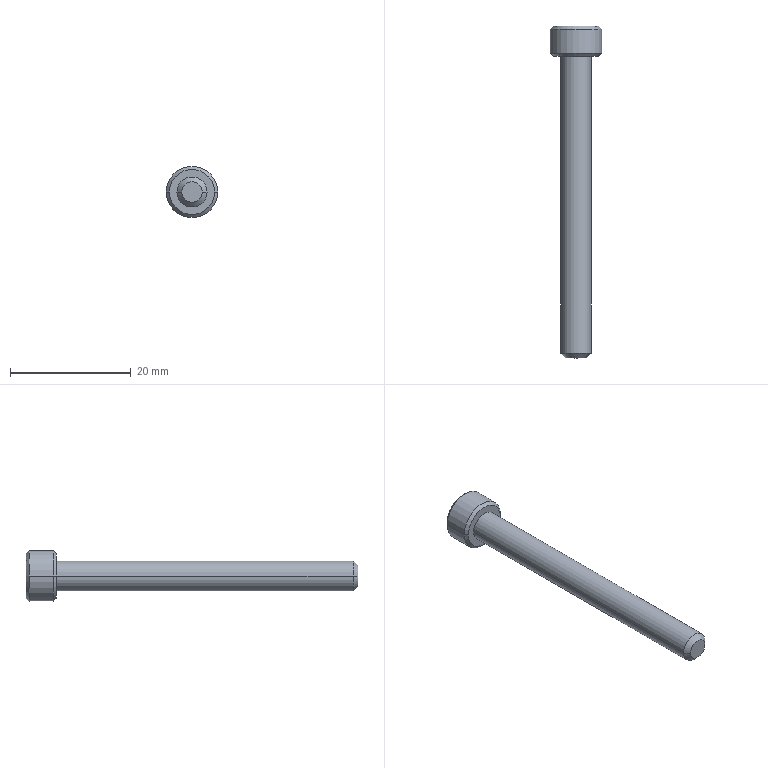Part | STEP file | BB62-M5-50L-14 | 1 solid | 27 faces | box 8.5 x 55 x 8.5 mm | volume 1213 mm3 | plane 15 | cone 8 | cylinder 4 | commonest cylinder face diameters 5 x2 8.5 x2
STEP:
#1=CARTESIAN_POINT('',(0.,1.178,0.));
#2=VERTEX_POINT('',#1);
#3=CARTESIAN_POINT('',(2.29,2.5,0.));
#4=VERTEX_POINT('',#3);
#5=CARTESIAN_POINT('',(0.,1.178,0.));
#6=DIRECTION('',(0.866,0.5,0.));
#7=VECTOR('',#6,1000.);
#8=LINE('',#5,#7);
#9=EDGE_CURVE('',#2,#4,#8,.T.);
#10=ORIENTED_EDGE('',*,*,#9,.F.);
#11=CARTESIAN_POINT('',(-2.29,2.5,0.));
#12=VERTEX_POINT('',#11);
#13=CARTESIAN_POINT('',(0.,1.178,0.));
#14=DIRECTION('',(-0.866,0.5,0.));
#15=VECTOR('',#14,1000.);
#16=LINE('',#13,#15);
#17=EDGE_CURVE('',#2,#12,#16,.T.);
#18=ORIENTED_EDGE('',*,*,#17,.T.);
#19=CARTESIAN_POINT('',(-1.983,2.5,1.145));
#20=VERTEX_POINT('',#19);
#21=CARTESIAN_POINT('',(0.,2.5,0.));
#22=DIRECTION('',(0.,-1.,0.));
#23=DIRECTION('',(-1.,0.,0.));
#24=AXIS2_PLACEMENT_3D('',#21,#22,#23);
#25=CIRCLE('',#24,2.29);
#26=EDGE_CURVE('',#20,#12,#25,.T.);
#27=ORIENTED_EDGE('',*,*,#26,.F.);
#28=CARTESIAN_POINT('',(0.,2.5,2.29));
#29=VERTEX_POINT('',#28);
#30=CARTESIAN_POINT('',(0.,2.5,0.));
#31=DIRECTION('',(0.,-1.,0.));
#32=DIRECTION('',(-1.,0.,0.));
#33=AXIS2_PLACEMENT_3D('',#30,#31,#32);
#34=CIRCLE('',#33,2.29);
#35=EDGE_CURVE('',#29,#20,#34,.T.);
#36=ORIENTED_EDGE('',*,*,#35,.F.);
#37=CARTESIAN_POINT('',(1.983,2.5,1.145));
#38=VERTEX_POINT('',#37);
#39=CARTESIAN_POINT('',(0.,2.5,0.));
#40=DIRECTION('',(0.,-1.,0.));
#41=DIRECTION('',(-1.,0.,0.));
#42=AXIS2_PLACEMENT_3D('',#39,#40,#41);
#43=CIRCLE('',#42,2.29);
#44=EDGE_CURVE('',#38,#29,#43,.T.);
#45=ORIENTED_EDGE('',*,*,#44,.F.);
#46=CARTESIAN_POINT('',(0.,2.5,0.));
#47=DIRECTION('',(0.,-1.,0.));
#48=DIRECTION('',(-1.,0.,0.));
#49=AXIS2_PLACEMENT_3D('',#46,#47,#48);
#50=CIRCLE('',#49,2.29);
#51=EDGE_CURVE('',#4,#38,#50,.T.);
#52=ORIENTED_EDGE('',*,*,#51,.F.);
#53=EDGE_LOOP('',(#10,#18,#27,#36,#45,#52));
#54=FACE_OUTER_BOUND('',#53,.T.);
#55=CARTESIAN_POINT('',(0.,1001.178,0.));
#56=DIRECTION('',(0.,1.,0.));
#57=DIRECTION('',(1.,0.,0.));
#58=AXIS2_PLACEMENT_3D('',#55,#56,#57);
#59=CONICAL_SURFACE('',#58,1732.051,1.047);
#60=ADVANCED_FACE('',(#54),#59,.F.);
#61=CARTESIAN_POINT('',(1.7,-50.,0.));
#62=VERTEX_POINT('',#61);
#63=CARTESIAN_POINT('',(-1.7,-50.,0.));
#64=VERTEX_POINT('',#63);
#65=CARTESIAN_POINT('',(0.,-50.,0.));
#66=DIRECTION('',(0.,1.,0.));
#67=DIRECTION('',(1.,0.,0.));
#68=AXIS2_PLACEMENT_3D('',#65,#66,#67);
#69=CIRCLE('',#68,1.7);
#70=EDGE_CURVE('',#62,#64,#69,.T.);
#71=ORIENTED_EDGE('',*,*,#70,.T.);
#72=CARTESIAN_POINT('',(-2.5,-49.2,0.));
#73=VERTEX_POINT('',#72);
#74=CARTESIAN_POINT('',(-1.7,-50.,0.));
#75=DIRECTION('',(-0.7071,0.7071,0.));
#76=VECTOR('',#75,1000.);
#77=LINE('',#74,#76);
#78=EDGE_CURVE('',#64,#73,#77,.T.);
#79=ORIENTED_EDGE('',*,*,#78,.T.);
#80=CARTESIAN_POINT('',(2.5,-49.2,0.));
#81=VERTEX_POINT('',#80);
#82=CARTESIAN_POINT('',(0.,-49.2,0.));
#83=DIRECTION('',(0.,-1.,0.));
#84=DIRECTION('',(-1.,0.,0.));
#85=AXIS2_PLACEMENT_3D('',#82,#83,#84);
#86=CIRCLE('',#85,2.5);
#87=EDGE_CURVE('',#73,#81,#86,.T.);
#88=ORIENTED_EDGE('',*,*,#87,.T.);
#89=CARTESIAN_POINT('',(1.7,-50.,0.));
#90=DIRECTION('',(0.7071,0.7071,0.));
#91=VECTOR('',#90,1000.);
#92=LINE('',#89,#91);
#93=EDGE_CURVE('',#62,#81,#92,.T.);
#94=ORIENTED_EDGE('',*,*,#93,.F.);
#95=EDGE_LOOP('',(#71,#79,#88,#94));
#96=FACE_OUTER_BOUND('',#95,.T.);
#97=CARTESIAN_POINT('',(0.,-50.,0.));
#98=DIRECTION('',(0.,1.,0.));
#99=DIRECTION('',(1.,0.,0.));
#100=AXIS2_PLACEMENT_3D('',#97,#98,#99);
#101=CONICAL_SURFACE('',#100,1.7,0.7854);
#102=ADVANCED_FACE('',(#96),#101,.T.);
#103=ORIENTED_EDGE('',*,*,#87,.F.);
#104=CARTESIAN_POINT('',(-2.5,0.,0.));
#105=VERTEX_POINT('',#104);
#106=CARTESIAN_POINT('',(-2.5,-49.2,0.));
#107=DIRECTION('',(0.,1.,0.));
#108=VECTOR('',#107,1000.);
#109=LINE('',#106,#108);
#110=EDGE_CURVE('',#73,#105,#109,.T.);
#111=ORIENTED_EDGE('',*,*,#110,.T.);
#112=CARTESIAN_POINT('',(2.5,0.,0.));
#113=VERTEX_POINT('',#112);
#114=CARTESIAN_POINT('',(0.,0.,0.));
#115=DIRECTION('',(0.,-1.,0.));
#116=DIRECTION('',(-1.,0.,0.));
#117=AXIS2_PLACEMENT_3D('',#114,#115,#116);
#118=CIRCLE('',#117,2.5);
#119=EDGE_CURVE('',#105,#113,#118,.T.);
#120=ORIENTED_EDGE('',*,*,#119,.T.);
#121=CARTESIAN_POINT('',(2.5,-49.2,0.));
#122=DIRECTION('',(0.,1.,0.));
#123=VECTOR('',#122,1000.);
#124=LINE('',#121,#123);
#125=EDGE_CURVE('',#81,#113,#124,.T.);
#126=ORIENTED_EDGE('',*,*,#125,.F.);
#127=EDGE_LOOP('',(#103,#111,#120,#126));
#128=FACE_OUTER_BOUND('',#127,.T.);
#129=CARTESIAN_POINT('',(0.,-49.2,0.));
#130=DIRECTION('',(0.,1.,0.));
#131=DIRECTION('',(1.,0.,0.));
#132=AXIS2_PLACEMENT_3D('',#129,#130,#131);
#133=CYLINDRICAL_SURFACE('',#132,2.5);
#134=ADVANCED_FACE('',(#128),#133,.T.);
#135=CARTESIAN_POINT('',(-3.75,5.,0.));
#136=VERTEX_POINT('',#135);
#137=CARTESIAN_POINT('',(3.75,5.,0.));
#138=VERTEX_POINT('',#137);
#139=CARTESIAN_POINT('',(0.,5.,0.));
#140=DIRECTION('',(0.,-1.,0.));
#141=DIRECTION('',(-1.,0.,0.));
#142=AXIS2_PLACEMENT_3D('',#139,#140,#141);
#143=CIRCLE('',#142,3.75);
#144=EDGE_CURVE('',#136,#138,#143,.T.);
#145=ORIENTED_EDGE('',*,*,#144,.T.);
#146=CARTESIAN_POINT('',(4.25,4.5,0.));
#147=VERTEX_POINT('',#146);
#148=CARTESIAN_POINT('',(4.25,4.5,0.));
#149=DIRECTION('',(0.7071,-0.7071,0.));
#150=VECTOR('',#149,1000.);
#151=LINE('',#148,#150);
#152=EDGE_CURVE('',#138,#147,#151,.T.);
#153=ORIENTED_EDGE('',*,*,#152,.T.);
#154=CARTESIAN_POINT('',(-4.25,4.5,0.));
#155=VERTEX_POINT('',#154);
#156=CARTESIAN_POINT('',(0.,4.5,0.));
#157=DIRECTION('',(0.,-1.,0.));
#158=DIRECTION('',(-1.,0.,0.));
#159=AXIS2_PLACEMENT_3D('',#156,#157,#158);
#160=CIRCLE('',#159,4.25);
#161=EDGE_CURVE('',#155,#147,#160,.T.);
#162=ORIENTED_EDGE('',*,*,#161,.F.);
#163=CARTESIAN_POINT('',(-4.25,4.5,0.));
#164=DIRECTION('',(-0.7071,-0.7071,0.));
#165=VECTOR('',#164,1000.);
#166=LINE('',#163,#165);
#167=EDGE_CURVE('',#136,#155,#166,.T.);
#168=ORIENTED_EDGE('',*,*,#167,.F.);
#169=EDGE_LOOP('',(#145,#153,#162,#168));
#170=FACE_OUTER_BOUND('',#169,.T.);
#171=CARTESIAN_POINT('',(0.,4.5,0.));
#172=DIRECTION('',(0.,-1.,0.));
#173=DIRECTION('',(-1.,0.,0.));
#174=AXIS2_PLACEMENT_3D('',#171,#172,#173);
#175=CONICAL_SURFACE('',#174,4.25,0.7854);
#176=ADVANCED_FACE('',(#170),#175,.T.);
#177=ORIENTED_EDGE('',*,*,#161,.T.);
#178=CARTESIAN_POINT('',(4.25,0.5,0.));
#179=VERTEX_POINT('',#178);
#180=CARTESIAN_POINT('',(4.25,1.62,0.));
#181=DIRECTION('',(0.,-1.,0.));
#182=VECTOR('',#181,1000.);
#183=LINE('',#180,#182);
#184=EDGE_CURVE('',#147,#179,#183,.T.);
#185=ORIENTED_EDGE('',*,*,#184,.T.);
#186=CARTESIAN_POINT('',(-4.25,0.5,0.));
#187=VERTEX_POINT('',#186);
#188=CARTESIAN_POINT('',(0.,0.5,0.));
#189=DIRECTION('',(0.,-1.,0.));
#190=DIRECTION('',(-1.,0.,0.));
#191=AXIS2_PLACEMENT_3D('',#188,#189,#190);
#192=CIRCLE('',#191,4.25);
#193=EDGE_CURVE('',#187,#179,#192,.T.);
#194=ORIENTED_EDGE('',*,*,#193,.F.);
#195=CARTESIAN_POINT('',(-4.25,1.62,0.));
#196=DIRECTION('',(0.,-1.,0.));
#197=VECTOR('',#196,1000.);
#198=LINE('',#195,#197);
#199=EDGE_CURVE('',#155,#187,#198,.T.);
#200=ORIENTED_EDGE('',*,*,#199,.F.);
#201=EDGE_LOOP('',(#177,#185,#194,#200));
#202=FACE_OUTER_BOUND('',#201,.T.);
#203=CARTESIAN_POINT('',(0.,1.62,0.));
#204=DIRECTION('',(0.,-1.,0.));
#205=DIRECTION('',(-1.,0.,0.));
#206=AXIS2_PLACEMENT_3D('',#203,#204,#205);
#207=CYLINDRICAL_SURFACE('',#206,4.25);
#208=ADVANCED_FACE('',(#202),#207,.T.);
#209=CARTESIAN_POINT('',(-3.75,0.,0.));
#210=VERTEX_POINT('',#209);
#211=CARTESIAN_POINT('',(3.75,0.,0.));
#212=VERTEX_POINT('',#211);
#213=CARTESIAN_POINT('',(0.,0.,0.));
#214=DIRECTION('',(0.,-1.,0.));
#215=DIRECTION('',(-1.,0.,0.));
#216=AXIS2_PLACEMENT_3D('',#213,#214,#215);
#217=CIRCLE('',#216,3.75);
#218=EDGE_CURVE('',#210,#212,#217,.T.);
#219=ORIENTED_EDGE('',*,*,#218,.F.);
#220=CARTESIAN_POINT('',(-3.75,0.,0.));
#221=DIRECTION('',(-0.7071,0.7071,0.));
#222=VECTOR('',#221,1000.);
#223=LINE('',#220,#222);
#224=EDGE_CURVE('',#210,#187,#223,.T.);
#225=ORIENTED_EDGE('',*,*,#224,.T.);
#226=ORIENTED_EDGE('',*,*,#193,.T.);
#227=CARTESIAN_POINT('',(3.75,0.,0.));
#228=DIRECTION('',(0.7071,0.7071,0.));
#229=VECTOR('',#228,1000.);
#230=LINE('',#227,#229);
#231=EDGE_CURVE('',#212,#179,#230,.T.);
#232=ORIENTED_EDGE('',*,*,#231,.F.);
#233=EDGE_LOOP('',(#219,#225,#226,#232));
#234=FACE_OUTER_BOUND('',#233,.T.);
#235=CARTESIAN_POINT('',(0.,0.,0.));
#236=DIRECTION('',(0.,1.,0.));
#237=DIRECTION('',(1.,0.,0.));
#238=AXIS2_PLACEMENT_3D('',#235,#236,#237);
#239=CONICAL_SURFACE('',#238,3.75,0.7854);
#240=ADVANCED_FACE('',(#234),#239,.T.);
#241=ORIENTED_EDGE('',*,*,#144,.F.);
#242=CARTESIAN_POINT('',(0.,5.,0.));
#243=DIRECTION('',(0.,-1.,0.));
#244=DIRECTION('',(-1.,0.,0.));
#245=AXIS2_PLACEMENT_3D('',#242,#243,#244);
#246=CIRCLE('',#245,3.75);
#247=EDGE_CURVE('',#138,#136,#246,.T.);
#248=ORIENTED_EDGE('',*,*,#247,.F.);
#249=EDGE_LOOP('',(#241,#248));
#250=FACE_OUTER_BOUND('',#249,.T.);
#251=CARTESIAN_POINT('',(0.,5.,-2.29));
#252=VERTEX_POINT('',#251);
#253=CARTESIAN_POINT('',(-1.983,5.,-1.145));
#254=VERTEX_POINT('',#253);
#255=CARTESIAN_POINT('',(0.,5.,-2.29));
#256=DIRECTION('',(-0.866,0.,0.5));
#257=VECTOR('',#256,1000.);
#258=LINE('',#255,#257);
#259=EDGE_CURVE('',#252,#254,#258,.T.);
#260=ORIENTED_EDGE('',*,*,#259,.F.);
#261=CARTESIAN_POINT('',(1.983,5.,-1.145));
#262=VERTEX_POINT('',#261);
#263=CARTESIAN_POINT('',(1.983,5.,-1.145));
#264=DIRECTION('',(-0.866,0.,-0.5));
#265=VECTOR('',#264,1000.);
#266=LINE('',#263,#265);
#267=EDGE_CURVE('',#262,#252,#266,.T.);
#268=ORIENTED_EDGE('',*,*,#267,.F.);
#269=CARTESIAN_POINT('',(1.983,5.,1.145));
#270=VERTEX_POINT('',#269);
#271=CARTESIAN_POINT('',(1.983,5.,1.145));
#272=DIRECTION('',(0.,0.,-1.));
#273=VECTOR('',#272,1000.);
#274=LINE('',#271,#273);
#275=EDGE_CURVE('',#270,#262,#274,.T.);
#276=ORIENTED_EDGE('',*,*,#275,.F.);
#277=CARTESIAN_POINT('',(0.,5.,2.29));
#278=VERTEX_POINT('',#277);
#279=CARTESIAN_POINT('',(0.,5.,2.29));
#280=DIRECTION('',(0.866,0.,-0.5));
#281=VECTOR('',#280,1000.);
#282=LINE('',#279,#281);
#283=EDGE_CURVE('',#278,#270,#282,.T.);
#284=ORIENTED_EDGE('',*,*,#283,.F.);
#285=CARTESIAN_POINT('',(-1.983,5.,1.145));
#286=VERTEX_POINT('',#285);
#287=CARTESIAN_POINT('',(-1.983,5.,1.145));
#288=DIRECTION('',(0.866,0.,0.5));
#289=VECTOR('',#288,1000.);
#290=LINE('',#287,#289);
#291=EDGE_CURVE('',#286,#278,#290,.T.);
#292=ORIENTED_EDGE('',*,*,#291,.F.);
#293=CARTESIAN_POINT('',(-1.983,5.,-1.145));
#294=DIRECTION('',(0.,0.,1.));
#295=VECTOR('',#294,1000.);
#296=LINE('',#293,#295);
#297=EDGE_CURVE('',#254,#286,#296,.T.);
#298=ORIENTED_EDGE('',*,*,#297,.F.);
#299=EDGE_LOOP('',(#260,#268,#276,#284,#292,#298));
#300=FACE_BOUND('',#299,.T.);
#301=CARTESIAN_POINT('',(3.75,5.,0.));
#302=DIRECTION('',(0.,1.,0.));
#303=DIRECTION('',(1.,0.,0.));
#304=AXIS2_PLACEMENT_3D('',#301,#302,#303);
#305=PLANE('',#304);
#306=ADVANCED_FACE('',(#250,#300),#305,.T.);
#307=CARTESIAN_POINT('',(0.,0.,0.));
#308=DIRECTION('',(0.,-1.,0.));
#309=DIRECTION('',(-1.,0.,0.));
#310=AXIS2_PLACEMENT_3D('',#307,#308,#309);
#311=CIRCLE('',#310,2.5);
#312=EDGE_CURVE('',#113,#105,#311,.T.);
#313=ORIENTED_EDGE('',*,*,#312,.F.);
#314=ORIENTED_EDGE('',*,*,#119,.F.);
#315=EDGE_LOOP('',(#313,#314));
#316=FACE_BOUND('',#315,.T.);
#317=CARTESIAN_POINT('',(0.,0.,0.));
#318=DIRECTION('',(0.,-1.,0.));
#319=DIRECTION('',(-1.,0.,0.));
#320=AXIS2_PLACEMENT_3D('',#317,#318,#319);
#321=CIRCLE('',#320,3.75);
#322=EDGE_CURVE('',#212,#210,#321,.T.);
#323=ORIENTED_EDGE('',*,*,#322,.T.);
#324=ORIENTED_EDGE('',*,*,#218,.T.);
#325=EDGE_LOOP('',(#323,#324));
#326=FACE_OUTER_BOUND('',#325,.T.);
#327=CARTESIAN_POINT('',(0.,0.,0.));
#328=DIRECTION('',(0.,-1.,0.));
#329=DIRECTION('',(-1.,0.,0.));
#330=AXIS2_PLACEMENT_3D('',#327,#328,#329);
#331=PLANE('',#330);
#332=ADVANCED_FACE('',(#316,#326),#331,.T.);
#333=ORIENTED_EDGE('',*,*,#224,.F.);
#334=ORIENTED_EDGE('',*,*,#322,.F.);
#335=ORIENTED_EDGE('',*,*,#231,.T.);
#336=CARTESIAN_POINT('',(0.,0.5,0.));
#337=DIRECTION('',(0.,-1.,0.));
#338=DIRECTION('',(-1.,0.,0.));
#339=AXIS2_PLACEMENT_3D('',#336,#337,#338);
#340=CIRCLE('',#339,4.25);
#341=EDGE_CURVE('',#179,#187,#340,.T.);
#342=ORIENTED_EDGE('',*,*,#341,.T.);
#343=EDGE_LOOP('',(#333,#334,#335,#342));
#344=FACE_OUTER_BOUND('',#343,.T.);
#345=CARTESIAN_POINT('',(0.,0.,0.));
#346=DIRECTION('',(0.,1.,0.));
#347=DIRECTION('',(1.,0.,0.));
#348=AXIS2_PLACEMENT_3D('',#345,#346,#347);
#349=CONICAL_SURFACE('',#348,3.75,0.7854);
#350=ADVANCED_FACE('',(#344),#349,.T.);
#351=ORIENTED_EDGE('',*,*,#184,.F.);
#352=CARTESIAN_POINT('',(0.,4.5,0.));
#353=DIRECTION('',(0.,-1.,0.));
#354=DIRECTION('',(-1.,0.,0.));
#355=AXIS2_PLACEMENT_3D('',#352,#353,#354);
#356=CIRCLE('',#355,4.25);
#357=EDGE_CURVE('',#147,#155,#356,.T.);
#358=ORIENTED_EDGE('',*,*,#357,.T.);
#359=ORIENTED_EDGE('',*,*,#199,.T.);
#360=ORIENTED_EDGE('',*,*,#341,.F.);
#361=EDGE_LOOP('',(#351,#358,#359,#360));
#362=FACE_OUTER_BOUND('',#361,.T.);
#363=CARTESIAN_POINT('',(0.,1.62,0.));
#364=DIRECTION('',(0.,-1.,0.));
#365=DIRECTION('',(-1.,0.,0.));
#366=AXIS2_PLACEMENT_3D('',#363,#364,#365);
#367=CYLINDRICAL_SURFACE('',#366,4.25);
#368=ADVANCED_FACE('',(#362),#367,.T.);
#369=ORIENTED_EDGE('',*,*,#152,.F.);
#370=ORIENTED_EDGE('',*,*,#247,.T.);
#371=ORIENTED_EDGE('',*,*,#167,.T.);
#372=ORIENTED_EDGE('',*,*,#357,.F.);
#373=EDGE_LOOP('',(#369,#370,#371,#372));
#374=FACE_OUTER_BOUND('',#373,.T.);
#375=CARTESIAN_POINT('',(0.,4.5,0.));
#376=DIRECTION('',(0.,-1.,0.));
#377=DIRECTION('',(-1.,0.,0.));
#378=AXIS2_PLACEMENT_3D('',#375,#376,#377);
#379=CONICAL_SURFACE('',#378,4.25,0.7854);
#380=ADVANCED_FACE('',(#374),#379,.T.);
#381=ORIENTED_EDGE('',*,*,#110,.F.);
#382=CARTESIAN_POINT('',(0.,-49.2,0.));
#383=DIRECTION('',(0.,-1.,0.));
#384=DIRECTION('',(-1.,0.,0.));
#385=AXIS2_PLACEMENT_3D('',#382,#383,#384);
#386=CIRCLE('',#385,2.5);
#387=EDGE_CURVE('',#81,#73,#386,.T.);
#388=ORIENTED_EDGE('',*,*,#387,.F.);
#389=ORIENTED_EDGE('',*,*,#125,.T.);
#390=ORIENTED_EDGE('',*,*,#312,.T.);
#391=EDGE_LOOP('',(#381,#388,#389,#390));
#392=FACE_OUTER_BOUND('',#391,.T.);
#393=CARTESIAN_POINT('',(0.,-49.2,0.));
#394=DIRECTION('',(0.,1.,0.));
#395=DIRECTION('',(1.,0.,0.));
#396=AXIS2_PLACEMENT_3D('',#393,#394,#395);
#397=CYLINDRICAL_SURFACE('',#396,2.5);
#398=ADVANCED_FACE('',(#392),#397,.T.);
#399=ORIENTED_EDGE('',*,*,#70,.F.);
#400=CARTESIAN_POINT('',(0.,-50.,0.));
#401=DIRECTION('',(0.,1.,0.));
#402=DIRECTION('',(1.,0.,0.));
#403=AXIS2_PLACEMENT_3D('',#400,#401,#402);
#404=CIRCLE('',#403,1.7);
#405=EDGE_CURVE('',#64,#62,#404,.T.);
#406=ORIENTED_EDGE('',*,*,#405,.F.);
#407=EDGE_LOOP('',(#399,#406));
#408=FACE_OUTER_BOUND('',#407,.T.);
#409=CARTESIAN_POINT('',(0.,-50.,0.));
#410=DIRECTION('',(0.,-1.,0.));
#411=DIRECTION('',(-1.,0.,0.));
#412=AXIS2_PLACEMENT_3D('',#409,#410,#411);
#413=PLANE('',#412);
#414=ADVANCED_FACE('',(#408),#413,.T.);
#415=ORIENTED_EDGE('',*,*,#78,.F.);
#416=ORIENTED_EDGE('',*,*,#405,.T.);
#417=ORIENTED_EDGE('',*,*,#93,.T.);
#418=ORIENTED_EDGE('',*,*,#387,.T.);
#419=EDGE_LOOP('',(#415,#416,#417,#418));
#420=FACE_OUTER_BOUND('',#419,.T.);
#421=CARTESIAN_POINT('',(0.,-50.,0.));
#422=DIRECTION('',(0.,1.,0.));
#423=DIRECTION('',(1.,0.,0.));
#424=AXIS2_PLACEMENT_3D('',#421,#422,#423);
#425=CONICAL_SURFACE('',#424,1.7,0.7854);
#426=ADVANCED_FACE('',(#420),#425,.T.);
#427=CARTESIAN_POINT('',(1.983,2.5,-1.145));
#428=VERTEX_POINT('',#427);
#429=CARTESIAN_POINT('',(0.,2.5,-2.29));
#430=VERTEX_POINT('',#429);
#431=CARTESIAN_POINT('',(1.983,2.5,-1.145));
#432=DIRECTION('',(-0.866,0.,-0.5));
#433=VECTOR('',#432,1000.);
#434=LINE('',#431,#433);
#435=EDGE_CURVE('',#428,#430,#434,.T.);
#436=ORIENTED_EDGE('',*,*,#435,.F.);
#437=CARTESIAN_POINT('',(1.983,5.,-1.145));
#438=DIRECTION('',(0.,-1.,0.));
#439=VECTOR('',#438,1000.);
#440=LINE('',#437,#439);
#441=EDGE_CURVE('',#262,#428,#440,.T.);
#442=ORIENTED_EDGE('',*,*,#441,.F.);
#443=ORIENTED_EDGE('',*,*,#267,.T.);
#444=CARTESIAN_POINT('',(0.,5.,-2.29));
#445=DIRECTION('',(0.,-1.,0.));
#446=VECTOR('',#445,1000.);
#447=LINE('',#444,#446);
#448=EDGE_CURVE('',#252,#430,#447,.T.);
#449=ORIENTED_EDGE('',*,*,#448,.T.);
#450=EDGE_LOOP('',(#436,#442,#443,#449));
#451=FACE_OUTER_BOUND('',#450,.T.);
#452=CARTESIAN_POINT('',(1.983,5.,-1.145));
#453=DIRECTION('',(-0.5,0.,0.866));
#454=DIRECTION('',(0.866,0.,0.5));
#455=AXIS2_PLACEMENT_3D('',#452,#453,#454);
#456=PLANE('',#455);
#457=ADVANCED_FACE('',(#451),#456,.T.);
#458=CARTESIAN_POINT('',(-1.983,2.5,-1.145));
#459=VERTEX_POINT('',#458);
#460=CARTESIAN_POINT('',(0.,2.5,-2.29));
#461=DIRECTION('',(-0.866,0.,0.5));
#462=VECTOR('',#461,1000.);
#463=LINE('',#460,#462);
#464=EDGE_CURVE('',#430,#459,#463,.T.);
#465=ORIENTED_EDGE('',*,*,#464,.F.);
#466=ORIENTED_EDGE('',*,*,#448,.F.);
#467=ORIENTED_EDGE('',*,*,#259,.T.);
#468=CARTESIAN_POINT('',(-1.983,5.,-1.145));
#469=DIRECTION('',(0.,-1.,0.));
#470=VECTOR('',#469,1000.);
#471=LINE('',#468,#470);
#472=EDGE_CURVE('',#254,#459,#471,.T.);
#473=ORIENTED_EDGE('',*,*,#472,.T.);
#474=EDGE_LOOP('',(#465,#466,#467,#473));
#475=FACE_OUTER_BOUND('',#474,.T.);
#476=CARTESIAN_POINT('',(0.,5.,-2.29));
#477=DIRECTION('',(0.5,0.,0.866));
#478=DIRECTION('',(0.866,0.,-0.5));
#479=AXIS2_PLACEMENT_3D('',#476,#477,#478);
#480=PLANE('',#479);
#481=ADVANCED_FACE('',(#475),#480,.T.);
#482=CARTESIAN_POINT('',(-1.983,2.5,-1.145));
#483=DIRECTION('',(0.,0.,1.));
#484=VECTOR('',#483,1000.);
#485=LINE('',#482,#484);
#486=EDGE_CURVE('',#459,#20,#485,.T.);
#487=ORIENTED_EDGE('',*,*,#486,.F.);
#488=ORIENTED_EDGE('',*,*,#472,.F.);
#489=ORIENTED_EDGE('',*,*,#297,.T.);
#490=CARTESIAN_POINT('',(-1.983,5.,1.145));
#491=DIRECTION('',(0.,-1.,0.));
#492=VECTOR('',#491,1000.);
#493=LINE('',#490,#492);
#494=EDGE_CURVE('',#286,#20,#493,.T.);
#495=ORIENTED_EDGE('',*,*,#494,.T.);
#496=EDGE_LOOP('',(#487,#488,#489,#495));
#497=FACE_OUTER_BOUND('',#496,.T.);
#498=CARTESIAN_POINT('',(-1.983,5.,-1.145));
#499=DIRECTION('',(1.,0.,0.));
#500=DIRECTION('',(0.,0.,-1.));
#501=AXIS2_PLACEMENT_3D('',#498,#499,#500);
#502=PLANE('',#501);
#503=ADVANCED_FACE('',(#497),#502,.T.);
#504=CARTESIAN_POINT('',(-1.983,2.5,1.145));
#505=DIRECTION('',(0.866,0.,0.5));
#506=VECTOR('',#505,1000.);
#507=LINE('',#504,#506);
#508=EDGE_CURVE('',#20,#29,#507,.T.);
#509=ORIENTED_EDGE('',*,*,#508,.F.);
#510=ORIENTED_EDGE('',*,*,#494,.F.);
#511=ORIENTED_EDGE('',*,*,#291,.T.);
#512=CARTESIAN_POINT('',(0.,5.,2.29));
#513=DIRECTION('',(0.,-1.,0.));
#514=VECTOR('',#513,1000.);
#515=LINE('',#512,#514);
#516=EDGE_CURVE('',#278,#29,#515,.T.);
#517=ORIENTED_EDGE('',*,*,#516,.T.);
#518=EDGE_LOOP('',(#509,#510,#511,#517));
#519=FACE_OUTER_BOUND('',#518,.T.);
#520=CARTESIAN_POINT('',(-1.983,5.,1.145));
#521=DIRECTION('',(0.5,0.,-0.866));
#522=DIRECTION('',(-0.866,0.,-0.5));
#523=AXIS2_PLACEMENT_3D('',#520,#521,#522);
#524=PLANE('',#523);
#525=ADVANCED_FACE('',(#519),#524,.T.);
#526=CARTESIAN_POINT('',(0.,2.5,2.29));
#527=DIRECTION('',(0.866,0.,-0.5));
#528=VECTOR('',#527,1000.);
#529=LINE('',#526,#528);
#530=EDGE_CURVE('',#29,#38,#529,.T.);
#531=ORIENTED_EDGE('',*,*,#530,.F.);
#532=ORIENTED_EDGE('',*,*,#516,.F.);
#533=ORIENTED_EDGE('',*,*,#283,.T.);
#534=CARTESIAN_POINT('',(1.983,5.,1.145));
#535=DIRECTION('',(0.,-1.,0.));
#536=VECTOR('',#535,1000.);
#537=LINE('',#534,#536);
#538=EDGE_CURVE('',#270,#38,#537,.T.);
#539=ORIENTED_EDGE('',*,*,#538,.T.);
#540=EDGE_LOOP('',(#531,#532,#533,#539));
#541=FACE_OUTER_BOUND('',#540,.T.);
#542=CARTESIAN_POINT('',(0.,5.,2.29));
#543=DIRECTION('',(-0.5,0.,-0.866));
#544=DIRECTION('',(-0.866,0.,0.5));
#545=AXIS2_PLACEMENT_3D('',#542,#543,#544);
#546=PLANE('',#545);
#547=ADVANCED_FACE('',(#541),#546,.T.);
#548=CARTESIAN_POINT('',(1.983,2.5,1.145));
#549=DIRECTION('',(0.,0.,-1.));
#550=VECTOR('',#549,1000.);
#551=LINE('',#548,#550);
#552=EDGE_CURVE('',#38,#428,#551,.T.);
#553=ORIENTED_EDGE('',*,*,#552,.F.);
#554=ORIENTED_EDGE('',*,*,#538,.F.);
#555=ORIENTED_EDGE('',*,*,#275,.T.);
#556=ORIENTED_EDGE('',*,*,#441,.T.);
#557=EDGE_LOOP('',(#553,#554,#555,#556));
#558=FACE_OUTER_BOUND('',#557,.T.);
#559=CARTESIAN_POINT('',(1.983,5.,1.145));
#560=DIRECTION('',(-1.,0.,0.));
#561=DIRECTION('',(0.,0.,1.));
#562=AXIS2_PLACEMENT_3D('',#559,#560,#561);
#563=PLANE('',#562);
#564=ADVANCED_FACE('',(#558),#563,.T.);
#565=ORIENTED_EDGE('',*,*,#435,.T.);
#566=CARTESIAN_POINT('',(0.,2.5,0.));
#567=DIRECTION('',(0.,-1.,0.));
#568=DIRECTION('',(-1.,0.,0.));
#569=AXIS2_PLACEMENT_3D('',#566,#567,#568);
#570=CIRCLE('',#569,2.29);
#571=EDGE_CURVE('',#430,#428,#570,.T.);
#572=ORIENTED_EDGE('',*,*,#571,.T.);
#573=EDGE_LOOP('',(#565,#572));
#574=FACE_OUTER_BOUND('',#573,.T.);
#575=CARTESIAN_POINT('',(0.,2.5,0.));
#576=DIRECTION('',(0.,1.,0.));
#577=DIRECTION('',(1.,0.,0.));
#578=AXIS2_PLACEMENT_3D('',#575,#576,#577);
#579=PLANE('',#578);
#580=ADVANCED_FACE('',(#574),#579,.F.);
#581=ORIENTED_EDGE('',*,*,#552,.T.);
#582=CARTESIAN_POINT('',(0.,2.5,0.));
#583=DIRECTION('',(0.,-1.,0.));
#584=DIRECTION('',(-1.,0.,0.));
#585=AXIS2_PLACEMENT_3D('',#582,#583,#584);
#586=CIRCLE('',#585,2.29);
#587=EDGE_CURVE('',#428,#4,#586,.T.);
#588=ORIENTED_EDGE('',*,*,#587,.T.);
#589=ORIENTED_EDGE('',*,*,#51,.T.);
#590=EDGE_LOOP('',(#581,#588,#589));
#591=FACE_OUTER_BOUND('',#590,.T.);
#592=CARTESIAN_POINT('',(0.,2.5,0.));
#593=DIRECTION('',(0.,1.,0.));
#594=DIRECTION('',(1.,0.,0.));
#595=AXIS2_PLACEMENT_3D('',#592,#593,#594);
#596=PLANE('',#595);
#597=ADVANCED_FACE('',(#591),#596,.F.);
#598=ORIENTED_EDGE('',*,*,#530,.T.);
#599=ORIENTED_EDGE('',*,*,#44,.T.);
#600=EDGE_LOOP('',(#598,#599));
#601=FACE_OUTER_BOUND('',#600,.T.);
#602=CARTESIAN_POINT('',(0.,2.5,0.));
#603=DIRECTION('',(0.,1.,0.));
#604=DIRECTION('',(1.,0.,0.));
#605=AXIS2_PLACEMENT_3D('',#602,#603,#604);
#606=PLANE('',#605);
#607=ADVANCED_FACE('',(#601),#606,.F.);
#608=ORIENTED_EDGE('',*,*,#508,.T.);
#609=ORIENTED_EDGE('',*,*,#35,.T.);
#610=EDGE_LOOP('',(#608,#609));
#611=FACE_OUTER_BOUND('',#610,.T.);
#612=CARTESIAN_POINT('',(0.,2.5,0.));
#613=DIRECTION('',(0.,1.,0.));
#614=DIRECTION('',(1.,0.,0.));
#615=AXIS2_PLACEMENT_3D('',#612,#613,#614);
#616=PLANE('',#615);
#617=ADVANCED_FACE('',(#611),#616,.F.);
#618=ORIENTED_EDGE('',*,*,#486,.T.);
#619=ORIENTED_EDGE('',*,*,#26,.T.);
#620=CARTESIAN_POINT('',(0.,2.5,0.));
#621=DIRECTION('',(0.,-1.,0.));
#622=DIRECTION('',(-1.,0.,0.));
#623=AXIS2_PLACEMENT_3D('',#620,#621,#622);
#624=CIRCLE('',#623,2.29);
#625=EDGE_CURVE('',#12,#459,#624,.T.);
#626=ORIENTED_EDGE('',*,*,#625,.T.);
#627=EDGE_LOOP('',(#618,#619,#626));
#628=FACE_OUTER_BOUND('',#627,.T.);
#629=CARTESIAN_POINT('',(0.,2.5,0.));
#630=DIRECTION('',(0.,1.,0.));
#631=DIRECTION('',(1.,0.,0.));
#632=AXIS2_PLACEMENT_3D('',#629,#630,#631);
#633=PLANE('',#632);
#634=ADVANCED_FACE('',(#628),#633,.F.);
#635=ORIENTED_EDGE('',*,*,#464,.T.);
#636=CARTESIAN_POINT('',(0.,2.5,0.));
#637=DIRECTION('',(0.,-1.,0.));
#638=DIRECTION('',(-1.,0.,0.));
#639=AXIS2_PLACEMENT_3D('',#636,#637,#638);
#640=CIRCLE('',#639,2.29);
#641=EDGE_CURVE('',#459,#430,#640,.T.);
#642=ORIENTED_EDGE('',*,*,#641,.T.);
#643=EDGE_LOOP('',(#635,#642));
#644=FACE_OUTER_BOUND('',#643,.T.);
#645=CARTESIAN_POINT('',(0.,2.5,0.));
#646=DIRECTION('',(0.,1.,0.));
#647=DIRECTION('',(1.,0.,0.));
#648=AXIS2_PLACEMENT_3D('',#645,#646,#647);
#649=PLANE('',#648);
#650=ADVANCED_FACE('',(#644),#649,.F.);
#651=ORIENTED_EDGE('',*,*,#17,.F.);
#652=ORIENTED_EDGE('',*,*,#9,.T.);
#653=ORIENTED_EDGE('',*,*,#587,.F.);
#654=ORIENTED_EDGE('',*,*,#571,.F.);
#655=ORIENTED_EDGE('',*,*,#641,.F.);
#656=ORIENTED_EDGE('',*,*,#625,.F.);
#657=EDGE_LOOP('',(#651,#652,#653,#654,#655,#656));
#658=FACE_OUTER_BOUND('',#657,.T.);
#659=CARTESIAN_POINT('',(0.,1001.178,0.));
#660=DIRECTION('',(0.,1.,0.));
#661=DIRECTION('',(1.,0.,0.));
#662=AXIS2_PLACEMENT_3D('',#659,#660,#661);
#663=CONICAL_SURFACE('',#662,1732.051,1.047);
#664=ADVANCED_FACE('',(#658),#663,.F.);
#665=CLOSED_SHELL('',(#60,#102,#134,#176,#208,#240,#306,#332,#350,#368,#380,#398,#414,#426,#457,#481,#503,#525,#547,#564,#580,#597,#607,#617,#634,#650,#664));
#666=MANIFOLD_SOLID_BREP('',#665);
#667=CARTESIAN_POINT('',(0.,0.,0.));
#668=DIRECTION('',(0.,0.,1.));
#669=DIRECTION('',(1.,0.,0.));
#670=AXIS2_PLACEMENT_3D('',#667,#668,#669);
#671=(LENGTH_UNIT()NAMED_UNIT(*)SI_UNIT(.MILLI.,.METRE.));
#672=UNCERTAINTY_MEASURE_WITH_UNIT(LENGTH_MEASURE(0.00001),#671,'','');
#673=(NAMED_UNIT(*)PLANE_ANGLE_UNIT()SI_UNIT($,.RADIAN.));
#674=(NAMED_UNIT(*)SI_UNIT($,.STERADIAN.)SOLID_ANGLE_UNIT());
#675=(GEOMETRIC_REPRESENTATION_CONTEXT(3)GLOBAL_UNCERTAINTY_ASSIGNED_CONTEXT((#672))GLOBAL_UNIT_ASSIGNED_CONTEXT((#671,#673,#674))REPRESENTATION_CONTEXT('',''));
#676=ADVANCED_BREP_SHAPE_REPRESENTATION('',(#666,#670),#675);